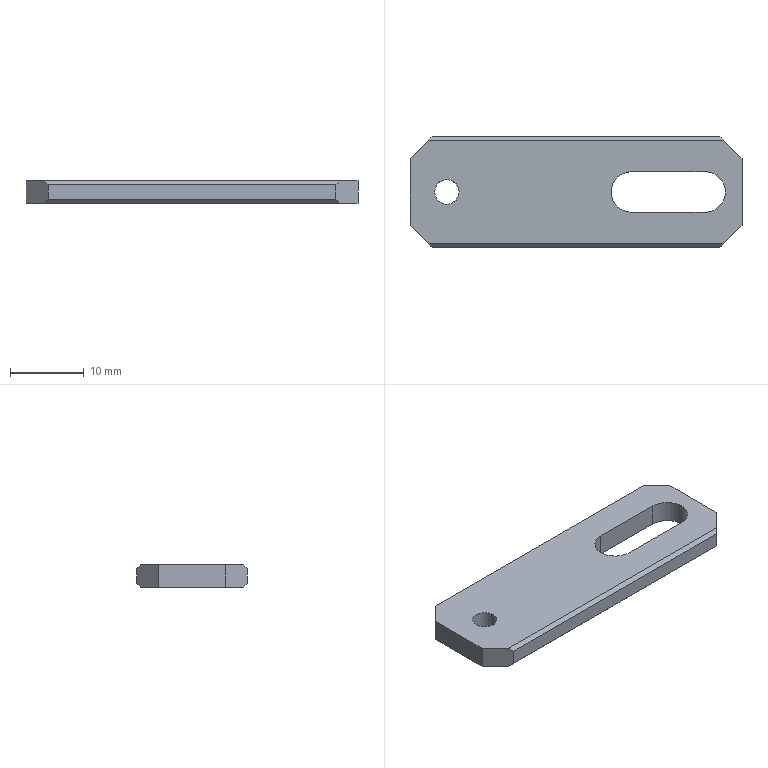Part | SolidWorks | features Chamfer 2, Extrusion 1, HoleWzd 1, ICE 1 | 1 solid | 21 faces | box 45 x 15 x 3 mm | volume 1689 mm3 | plane 16 | cylinder 5 | commonest cylinder face diameters 5.5 x3 3.3 x2
STEP:
#1=CARTESIAN_POINT('',(20.25,0.,0.));
#2=VERTEX_POINT('',#1);
#3=CARTESIAN_POINT('',(17.5,2.75,0.));
#4=VERTEX_POINT('',#3);
#5=CARTESIAN_POINT('',(17.5,0.,0.));
#6=DIRECTION('',(0.,0.,1.));
#7=DIRECTION('',(1.,0.,0.));
#8=AXIS2_PLACEMENT_3D('',#5,#6,#7);
#9=CIRCLE('',#8,2.75);
#10=EDGE_CURVE('',#2,#4,#9,.T.);
#11=ORIENTED_EDGE('',*,*,#10,.F.);
#12=CARTESIAN_POINT('',(20.25,0.,3.));
#13=VERTEX_POINT('',#12);
#14=CARTESIAN_POINT('',(20.25,0.,0.));
#15=DIRECTION('',(0.,0.,1.));
#16=VECTOR('',#15,1000.);
#17=LINE('',#14,#16);
#18=EDGE_CURVE('',#2,#13,#17,.T.);
#19=ORIENTED_EDGE('',*,*,#18,.T.);
#20=CARTESIAN_POINT('',(17.5,2.75,3.));
#21=VERTEX_POINT('',#20);
#22=CARTESIAN_POINT('',(17.5,0.,3.));
#23=DIRECTION('',(0.,0.,1.));
#24=DIRECTION('',(1.,0.,0.));
#25=AXIS2_PLACEMENT_3D('',#22,#23,#24);
#26=CIRCLE('',#25,2.75);
#27=EDGE_CURVE('',#13,#21,#26,.T.);
#28=ORIENTED_EDGE('',*,*,#27,.T.);
#29=CARTESIAN_POINT('',(17.5,2.75,0.));
#30=DIRECTION('',(0.,0.,1.));
#31=VECTOR('',#30,1000.);
#32=LINE('',#29,#31);
#33=EDGE_CURVE('',#4,#21,#32,.T.);
#34=ORIENTED_EDGE('',*,*,#33,.F.);
#35=EDGE_LOOP('',(#11,#19,#28,#34));
#36=FACE_OUTER_BOUND('',#35,.T.);
#37=CARTESIAN_POINT('',(17.5,0.,0.));
#38=DIRECTION('',(0.,0.,1.));
#39=DIRECTION('',(1.,0.,0.));
#40=AXIS2_PLACEMENT_3D('',#37,#38,#39);
#41=CYLINDRICAL_SURFACE('',#40,2.75);
#42=ADVANCED_FACE('',(#36),#41,.F.);
#43=CARTESIAN_POINT('',(-15.85,0.,0.));
#44=VERTEX_POINT('',#43);
#45=CARTESIAN_POINT('',(-19.15,0.,0.));
#46=VERTEX_POINT('',#45);
#47=CARTESIAN_POINT('',(-17.5,0.,0.));
#48=DIRECTION('',(0.,0.,-1.));
#49=DIRECTION('',(-1.,0.,0.));
#50=AXIS2_PLACEMENT_3D('',#47,#48,#49);
#51=CIRCLE('',#50,1.65);
#52=EDGE_CURVE('',#44,#46,#51,.T.);
#53=ORIENTED_EDGE('',*,*,#52,.T.);
#54=CARTESIAN_POINT('',(-19.15,0.,3.));
#55=VERTEX_POINT('',#54);
#56=CARTESIAN_POINT('',(-19.15,0.,3.));
#57=DIRECTION('',(0.,0.,1.));
#58=VECTOR('',#57,1000.);
#59=LINE('',#56,#58);
#60=EDGE_CURVE('',#46,#55,#59,.T.);
#61=ORIENTED_EDGE('',*,*,#60,.T.);
#62=CARTESIAN_POINT('',(-15.85,0.,3.));
#63=VERTEX_POINT('',#62);
#64=CARTESIAN_POINT('',(-17.5,0.,3.));
#65=DIRECTION('',(0.,0.,1.));
#66=DIRECTION('',(1.,0.,0.));
#67=AXIS2_PLACEMENT_3D('',#64,#65,#66);
#68=CIRCLE('',#67,1.65);
#69=EDGE_CURVE('',#55,#63,#68,.T.);
#70=ORIENTED_EDGE('',*,*,#69,.T.);
#71=CARTESIAN_POINT('',(-15.85,0.,3.));
#72=DIRECTION('',(0.,0.,1.));
#73=VECTOR('',#72,1000.);
#74=LINE('',#71,#73);
#75=EDGE_CURVE('',#44,#63,#74,.T.);
#76=ORIENTED_EDGE('',*,*,#75,.F.);
#77=EDGE_LOOP('',(#53,#61,#70,#76));
#78=FACE_OUTER_BOUND('',#77,.T.);
#79=CARTESIAN_POINT('',(-17.5,0.,3.));
#80=DIRECTION('',(0.,0.,1.));
#81=DIRECTION('',(1.,0.,0.));
#82=AXIS2_PLACEMENT_3D('',#79,#80,#81);
#83=CYLINDRICAL_SURFACE('',#82,1.65);
#84=ADVANCED_FACE('',(#78),#83,.F.);
#85=CARTESIAN_POINT('',(22.5,-4.5,3.));
#86=VERTEX_POINT('',#85);
#87=CARTESIAN_POINT('',(22.5,4.5,3.));
#88=VERTEX_POINT('',#87);
#89=CARTESIAN_POINT('',(22.5,-7.5,3.));
#90=DIRECTION('',(0.,1.,0.));
#91=VECTOR('',#90,1000.);
#92=LINE('',#89,#91);
#93=EDGE_CURVE('',#86,#88,#92,.T.);
#94=ORIENTED_EDGE('',*,*,#93,.F.);
#95=CARTESIAN_POINT('',(22.5,-4.5,0.));
#96=VERTEX_POINT('',#95);
#97=CARTESIAN_POINT('',(22.5,-4.5,3.));
#98=DIRECTION('',(0.,0.,-1.));
#99=VECTOR('',#98,1000.);
#100=LINE('',#97,#99);
#101=EDGE_CURVE('',#86,#96,#100,.T.);
#102=ORIENTED_EDGE('',*,*,#101,.T.);
#103=CARTESIAN_POINT('',(22.5,4.5,0.));
#104=VERTEX_POINT('',#103);
#105=CARTESIAN_POINT('',(22.5,-7.5,0.));
#106=DIRECTION('',(0.,1.,0.));
#107=VECTOR('',#106,1000.);
#108=LINE('',#105,#107);
#109=EDGE_CURVE('',#96,#104,#108,.T.);
#110=ORIENTED_EDGE('',*,*,#109,.T.);
#111=CARTESIAN_POINT('',(22.5,4.5,3.));
#112=DIRECTION('',(0.,0.,1.));
#113=VECTOR('',#112,1000.);
#114=LINE('',#111,#113);
#115=EDGE_CURVE('',#104,#88,#114,.T.);
#116=ORIENTED_EDGE('',*,*,#115,.T.);
#117=EDGE_LOOP('',(#94,#102,#110,#116));
#118=FACE_OUTER_BOUND('',#117,.T.);
#119=CARTESIAN_POINT('',(22.5,-7.5,3.));
#120=DIRECTION('',(-1.,0.,0.));
#121=DIRECTION('',(0.,0.,1.));
#122=AXIS2_PLACEMENT_3D('',#119,#120,#121);
#123=PLANE('',#122);
#124=ADVANCED_FACE('',(#118),#123,.F.);
#125=CARTESIAN_POINT('',(-19.5,7.5,0.5));
#126=VERTEX_POINT('',#125);
#127=CARTESIAN_POINT('',(-19.5,7.5,2.5));
#128=VERTEX_POINT('',#127);
#129=CARTESIAN_POINT('',(-19.5,7.5,3.));
#130=DIRECTION('',(0.,0.,1.));
#131=VECTOR('',#130,1000.);
#132=LINE('',#129,#131);
#133=EDGE_CURVE('',#126,#128,#132,.T.);
#134=ORIENTED_EDGE('',*,*,#133,.T.);
#135=CARTESIAN_POINT('',(19.5,7.5,2.5));
#136=VERTEX_POINT('',#135);
#137=CARTESIAN_POINT('',(-22.5,7.5,2.5));
#138=DIRECTION('',(1.,0.,0.));
#139=VECTOR('',#138,1000.);
#140=LINE('',#137,#139);
#141=EDGE_CURVE('',#128,#136,#140,.T.);
#142=ORIENTED_EDGE('',*,*,#141,.T.);
#143=CARTESIAN_POINT('',(19.5,7.5,0.5));
#144=VERTEX_POINT('',#143);
#145=CARTESIAN_POINT('',(19.5,7.5,3.));
#146=DIRECTION('',(0.,0.,-1.));
#147=VECTOR('',#146,1000.);
#148=LINE('',#145,#147);
#149=EDGE_CURVE('',#136,#144,#148,.T.);
#150=ORIENTED_EDGE('',*,*,#149,.T.);
#151=CARTESIAN_POINT('',(-19.5,7.5,0.5));
#152=DIRECTION('',(-1.,0.,0.));
#153=VECTOR('',#152,1000.);
#154=LINE('',#151,#153);
#155=EDGE_CURVE('',#144,#126,#154,.T.);
#156=ORIENTED_EDGE('',*,*,#155,.T.);
#157=EDGE_LOOP('',(#134,#142,#150,#156));
#158=FACE_OUTER_BOUND('',#157,.T.);
#159=CARTESIAN_POINT('',(-22.5,7.5,3.));
#160=DIRECTION('',(0.,-1.,0.));
#161=DIRECTION('',(0.,0.,-1.));
#162=AXIS2_PLACEMENT_3D('',#159,#160,#161);
#163=PLANE('',#162);
#164=ADVANCED_FACE('',(#158),#163,.F.);
#165=CARTESIAN_POINT('',(-22.5,4.5,0.));
#166=VERTEX_POINT('',#165);
#167=CARTESIAN_POINT('',(-22.5,-4.5,0.));
#168=VERTEX_POINT('',#167);
#169=CARTESIAN_POINT('',(-22.5,-7.5,0.));
#170=DIRECTION('',(0.,-1.,0.));
#171=VECTOR('',#170,1000.);
#172=LINE('',#169,#171);
#173=EDGE_CURVE('',#166,#168,#172,.T.);
#174=ORIENTED_EDGE('',*,*,#173,.T.);
#175=CARTESIAN_POINT('',(-22.5,-4.5,3.));
#176=VERTEX_POINT('',#175);
#177=CARTESIAN_POINT('',(-22.5,-4.5,3.));
#178=DIRECTION('',(0.,0.,1.));
#179=VECTOR('',#178,1000.);
#180=LINE('',#177,#179);
#181=EDGE_CURVE('',#168,#176,#180,.T.);
#182=ORIENTED_EDGE('',*,*,#181,.T.);
#183=CARTESIAN_POINT('',(-22.5,4.5,3.));
#184=VERTEX_POINT('',#183);
#185=CARTESIAN_POINT('',(-22.5,-7.5,3.));
#186=DIRECTION('',(0.,-1.,0.));
#187=VECTOR('',#186,1000.);
#188=LINE('',#185,#187);
#189=EDGE_CURVE('',#184,#176,#188,.T.);
#190=ORIENTED_EDGE('',*,*,#189,.F.);
#191=CARTESIAN_POINT('',(-22.5,4.5,3.));
#192=DIRECTION('',(0.,0.,-1.));
#193=VECTOR('',#192,1000.);
#194=LINE('',#191,#193);
#195=EDGE_CURVE('',#184,#166,#194,.T.);
#196=ORIENTED_EDGE('',*,*,#195,.T.);
#197=EDGE_LOOP('',(#174,#182,#190,#196));
#198=FACE_OUTER_BOUND('',#197,.T.);
#199=CARTESIAN_POINT('',(-22.5,-7.5,3.));
#200=DIRECTION('',(1.,0.,0.));
#201=DIRECTION('',(0.,0.,-1.));
#202=AXIS2_PLACEMENT_3D('',#199,#200,#201);
#203=PLANE('',#202);
#204=ADVANCED_FACE('',(#198),#203,.F.);
#205=CARTESIAN_POINT('',(19.5,-7.5,0.5));
#206=VERTEX_POINT('',#205);
#207=CARTESIAN_POINT('',(19.5,-7.5,2.5));
#208=VERTEX_POINT('',#207);
#209=CARTESIAN_POINT('',(19.5,-7.5,3.));
#210=DIRECTION('',(0.,0.,1.));
#211=VECTOR('',#210,1000.);
#212=LINE('',#209,#211);
#213=EDGE_CURVE('',#206,#208,#212,.T.);
#214=ORIENTED_EDGE('',*,*,#213,.T.);
#215=CARTESIAN_POINT('',(-19.5,-7.5,2.5));
#216=VERTEX_POINT('',#215);
#217=CARTESIAN_POINT('',(-22.5,-7.5,2.5));
#218=DIRECTION('',(-1.,0.,0.));
#219=VECTOR('',#218,1000.);
#220=LINE('',#217,#219);
#221=EDGE_CURVE('',#208,#216,#220,.T.);
#222=ORIENTED_EDGE('',*,*,#221,.T.);
#223=CARTESIAN_POINT('',(-19.5,-7.5,0.5));
#224=VERTEX_POINT('',#223);
#225=CARTESIAN_POINT('',(-19.5,-7.5,3.));
#226=DIRECTION('',(0.,0.,-1.));
#227=VECTOR('',#226,1000.);
#228=LINE('',#225,#227);
#229=EDGE_CURVE('',#216,#224,#228,.T.);
#230=ORIENTED_EDGE('',*,*,#229,.T.);
#231=CARTESIAN_POINT('',(19.5,-7.5,0.5));
#232=DIRECTION('',(1.,0.,0.));
#233=VECTOR('',#232,1000.);
#234=LINE('',#231,#233);
#235=EDGE_CURVE('',#224,#206,#234,.T.);
#236=ORIENTED_EDGE('',*,*,#235,.T.);
#237=EDGE_LOOP('',(#214,#222,#230,#236));
#238=FACE_OUTER_BOUND('',#237,.T.);
#239=CARTESIAN_POINT('',(-22.5,-7.5,3.));
#240=DIRECTION('',(0.,1.,0.));
#241=DIRECTION('',(0.,0.,1.));
#242=AXIS2_PLACEMENT_3D('',#239,#240,#241);
#243=PLANE('',#242);
#244=ADVANCED_FACE('',(#238),#243,.F.);
#245=CARTESIAN_POINT('',(7.5,-2.75,3.));
#246=VERTEX_POINT('',#245);
#247=CARTESIAN_POINT('',(17.5,-2.75,3.));
#248=VERTEX_POINT('',#247);
#249=CARTESIAN_POINT('',(7.5,-2.75,3.));
#250=DIRECTION('',(1.,0.,0.));
#251=VECTOR('',#250,1000.);
#252=LINE('',#249,#251);
#253=EDGE_CURVE('',#246,#248,#252,.T.);
#254=ORIENTED_EDGE('',*,*,#253,.F.);
#255=CARTESIAN_POINT('',(7.5,2.75,3.));
#256=VERTEX_POINT('',#255);
#257=CARTESIAN_POINT('',(7.5,0.,3.));
#258=DIRECTION('',(0.,0.,1.));
#259=DIRECTION('',(1.,0.,0.));
#260=AXIS2_PLACEMENT_3D('',#257,#258,#259);
#261=CIRCLE('',#260,2.75);
#262=EDGE_CURVE('',#256,#246,#261,.T.);
#263=ORIENTED_EDGE('',*,*,#262,.F.);
#264=CARTESIAN_POINT('',(7.5,2.75,3.));
#265=DIRECTION('',(-1.,0.,0.));
#266=VECTOR('',#265,1000.);
#267=LINE('',#264,#266);
#268=EDGE_CURVE('',#21,#256,#267,.T.);
#269=ORIENTED_EDGE('',*,*,#268,.F.);
#270=ORIENTED_EDGE('',*,*,#27,.F.);
#271=CARTESIAN_POINT('',(17.5,0.,3.));
#272=DIRECTION('',(0.,0.,1.));
#273=DIRECTION('',(1.,0.,0.));
#274=AXIS2_PLACEMENT_3D('',#271,#272,#273);
#275=CIRCLE('',#274,2.75);
#276=EDGE_CURVE('',#248,#13,#275,.T.);
#277=ORIENTED_EDGE('',*,*,#276,.F.);
#278=EDGE_LOOP('',(#254,#263,#269,#270,#277));
#279=FACE_BOUND('',#278,.T.);
#280=CARTESIAN_POINT('',(-17.5,0.,3.));
#281=DIRECTION('',(0.,0.,1.));
#282=DIRECTION('',(1.,0.,0.));
#283=AXIS2_PLACEMENT_3D('',#280,#281,#282);
#284=CIRCLE('',#283,1.65);
#285=EDGE_CURVE('',#63,#55,#284,.T.);
#286=ORIENTED_EDGE('',*,*,#285,.F.);
#287=ORIENTED_EDGE('',*,*,#69,.F.);
#288=EDGE_LOOP('',(#286,#287));
#289=FACE_BOUND('',#288,.T.);
#290=CARTESIAN_POINT('',(20.,7.,3.));
#291=VERTEX_POINT('',#290);
#292=CARTESIAN_POINT('',(19.5,7.5,3.));
#293=DIRECTION('',(-0.7071,0.7071,0.));
#294=VECTOR('',#293,1000.);
#295=LINE('',#292,#294);
#296=EDGE_CURVE('',#88,#291,#295,.T.);
#297=ORIENTED_EDGE('',*,*,#296,.T.);
#298=CARTESIAN_POINT('',(-20.,7.,3.));
#299=VERTEX_POINT('',#298);
#300=CARTESIAN_POINT('',(0.,7.,3.));
#301=DIRECTION('',(-1.,0.,0.));
#302=VECTOR('',#301,1000.);
#303=LINE('',#300,#302);
#304=EDGE_CURVE('',#291,#299,#303,.T.);
#305=ORIENTED_EDGE('',*,*,#304,.T.);
#306=CARTESIAN_POINT('',(-22.5,4.5,3.));
#307=DIRECTION('',(-0.7071,-0.7071,0.));
#308=VECTOR('',#307,1000.);
#309=LINE('',#306,#308);
#310=EDGE_CURVE('',#299,#184,#309,.T.);
#311=ORIENTED_EDGE('',*,*,#310,.T.);
#312=ORIENTED_EDGE('',*,*,#189,.T.);
#313=CARTESIAN_POINT('',(-20.,-7.,3.));
#314=VERTEX_POINT('',#313);
#315=CARTESIAN_POINT('',(-19.5,-7.5,3.));
#316=DIRECTION('',(0.7071,-0.7071,0.));
#317=VECTOR('',#316,1000.);
#318=LINE('',#315,#317);
#319=EDGE_CURVE('',#176,#314,#318,.T.);
#320=ORIENTED_EDGE('',*,*,#319,.T.);
#321=CARTESIAN_POINT('',(20.,-7.,3.));
#322=VERTEX_POINT('',#321);
#323=CARTESIAN_POINT('',(0.,-7.,3.));
#324=DIRECTION('',(1.,0.,0.));
#325=VECTOR('',#324,1000.);
#326=LINE('',#323,#325);
#327=EDGE_CURVE('',#314,#322,#326,.T.);
#328=ORIENTED_EDGE('',*,*,#327,.T.);
#329=CARTESIAN_POINT('',(22.5,-4.5,3.));
#330=DIRECTION('',(0.7071,0.7071,0.));
#331=VECTOR('',#330,1000.);
#332=LINE('',#329,#331);
#333=EDGE_CURVE('',#322,#86,#332,.T.);
#334=ORIENTED_EDGE('',*,*,#333,.T.);
#335=ORIENTED_EDGE('',*,*,#93,.T.);
#336=EDGE_LOOP('',(#297,#305,#311,#312,#320,#328,#334,#335));
#337=FACE_OUTER_BOUND('',#336,.T.);
#338=CARTESIAN_POINT('',(0.,0.,3.));
#339=DIRECTION('',(0.,0.,-1.));
#340=DIRECTION('',(-1.,0.,0.));
#341=AXIS2_PLACEMENT_3D('',#338,#339,#340);
#342=PLANE('',#341);
#343=ADVANCED_FACE('',(#279,#289,#337),#342,.F.);
#344=CARTESIAN_POINT('',(7.5,2.75,0.));
#345=VERTEX_POINT('',#344);
#346=CARTESIAN_POINT('',(7.5,-2.75,0.));
#347=VERTEX_POINT('',#346);
#348=CARTESIAN_POINT('',(7.5,0.,0.));
#349=DIRECTION('',(0.,0.,1.));
#350=DIRECTION('',(1.,0.,0.));
#351=AXIS2_PLACEMENT_3D('',#348,#349,#350);
#352=CIRCLE('',#351,2.75);
#353=EDGE_CURVE('',#345,#347,#352,.T.);
#354=ORIENTED_EDGE('',*,*,#353,.T.);
#355=CARTESIAN_POINT('',(17.5,-2.75,0.));
#356=VERTEX_POINT('',#355);
#357=CARTESIAN_POINT('',(7.5,-2.75,0.));
#358=DIRECTION('',(1.,0.,0.));
#359=VECTOR('',#358,1000.);
#360=LINE('',#357,#359);
#361=EDGE_CURVE('',#347,#356,#360,.T.);
#362=ORIENTED_EDGE('',*,*,#361,.T.);
#363=CARTESIAN_POINT('',(17.5,0.,0.));
#364=DIRECTION('',(0.,0.,1.));
#365=DIRECTION('',(1.,0.,0.));
#366=AXIS2_PLACEMENT_3D('',#363,#364,#365);
#367=CIRCLE('',#366,2.75);
#368=EDGE_CURVE('',#356,#2,#367,.T.);
#369=ORIENTED_EDGE('',*,*,#368,.T.);
#370=ORIENTED_EDGE('',*,*,#10,.T.);
#371=CARTESIAN_POINT('',(7.5,2.75,0.));
#372=DIRECTION('',(-1.,0.,0.));
#373=VECTOR('',#372,1000.);
#374=LINE('',#371,#373);
#375=EDGE_CURVE('',#4,#345,#374,.T.);
#376=ORIENTED_EDGE('',*,*,#375,.T.);
#377=EDGE_LOOP('',(#354,#362,#369,#370,#376));
#378=FACE_BOUND('',#377,.T.);
#379=ORIENTED_EDGE('',*,*,#52,.F.);
#380=CARTESIAN_POINT('',(-17.5,0.,0.));
#381=DIRECTION('',(0.,0.,-1.));
#382=DIRECTION('',(-1.,0.,0.));
#383=AXIS2_PLACEMENT_3D('',#380,#381,#382);
#384=CIRCLE('',#383,1.65);
#385=EDGE_CURVE('',#46,#44,#384,.T.);
#386=ORIENTED_EDGE('',*,*,#385,.F.);
#387=EDGE_LOOP('',(#379,#386));
#388=FACE_BOUND('',#387,.T.);
#389=CARTESIAN_POINT('',(-20.,7.,0.));
#390=VERTEX_POINT('',#389);
#391=CARTESIAN_POINT('',(-13.5,13.5,0.));
#392=DIRECTION('',(0.7071,0.7071,0.));
#393=VECTOR('',#392,1000.);
#394=LINE('',#391,#393);
#395=EDGE_CURVE('',#166,#390,#394,.T.);
#396=ORIENTED_EDGE('',*,*,#395,.T.);
#397=CARTESIAN_POINT('',(20.,7.,0.));
#398=VERTEX_POINT('',#397);
#399=CARTESIAN_POINT('',(19.5,7.,0.));
#400=DIRECTION('',(1.,0.,0.));
#401=VECTOR('',#400,1000.);
#402=LINE('',#399,#401);
#403=EDGE_CURVE('',#390,#398,#402,.T.);
#404=ORIENTED_EDGE('',*,*,#403,.T.);
#405=CARTESIAN_POINT('',(13.5,13.5,0.));
#406=DIRECTION('',(0.7071,-0.7071,0.));
#407=VECTOR('',#406,1000.);
#408=LINE('',#405,#407);
#409=EDGE_CURVE('',#398,#104,#408,.T.);
#410=ORIENTED_EDGE('',*,*,#409,.T.);
#411=ORIENTED_EDGE('',*,*,#109,.F.);
#412=CARTESIAN_POINT('',(20.,-7.,0.));
#413=VERTEX_POINT('',#412);
#414=CARTESIAN_POINT('',(13.5,-13.5,0.));
#415=DIRECTION('',(-0.7071,-0.7071,0.));
#416=VECTOR('',#415,1000.);
#417=LINE('',#414,#416);
#418=EDGE_CURVE('',#96,#413,#417,.T.);
#419=ORIENTED_EDGE('',*,*,#418,.T.);
#420=CARTESIAN_POINT('',(-20.,-7.,0.));
#421=VERTEX_POINT('',#420);
#422=CARTESIAN_POINT('',(-19.5,-7.,0.));
#423=DIRECTION('',(-1.,0.,0.));
#424=VECTOR('',#423,1000.);
#425=LINE('',#422,#424);
#426=EDGE_CURVE('',#413,#421,#425,.T.);
#427=ORIENTED_EDGE('',*,*,#426,.T.);
#428=CARTESIAN_POINT('',(-13.5,-13.5,0.));
#429=DIRECTION('',(-0.7071,0.7071,0.));
#430=VECTOR('',#429,1000.);
#431=LINE('',#428,#430);
#432=EDGE_CURVE('',#421,#168,#431,.T.);
#433=ORIENTED_EDGE('',*,*,#432,.T.);
#434=ORIENTED_EDGE('',*,*,#173,.F.);
#435=EDGE_LOOP('',(#396,#404,#410,#411,#419,#427,#433,#434));
#436=FACE_OUTER_BOUND('',#435,.T.);
#437=CARTESIAN_POINT('',(0.,0.,0.));
#438=DIRECTION('',(0.,0.,-1.));
#439=DIRECTION('',(-1.,0.,0.));
#440=AXIS2_PLACEMENT_3D('',#437,#438,#439);
#441=PLANE('',#440);
#442=ADVANCED_FACE('',(#378,#388,#436),#441,.T.);
#443=ORIENTED_EDGE('',*,*,#60,.F.);
#444=ORIENTED_EDGE('',*,*,#385,.T.);
#445=ORIENTED_EDGE('',*,*,#75,.T.);
#446=ORIENTED_EDGE('',*,*,#285,.T.);
#447=EDGE_LOOP('',(#443,#444,#445,#446));
#448=FACE_OUTER_BOUND('',#447,.T.);
#449=CARTESIAN_POINT('',(-17.5,0.,3.));
#450=DIRECTION('',(0.,0.,1.));
#451=DIRECTION('',(1.,0.,0.));
#452=AXIS2_PLACEMENT_3D('',#449,#450,#451);
#453=CYLINDRICAL_SURFACE('',#452,1.65);
#454=ADVANCED_FACE('',(#448),#453,.F.);
#455=ORIENTED_EDGE('',*,*,#262,.T.);
#456=CARTESIAN_POINT('',(7.5,-2.75,0.));
#457=DIRECTION('',(0.,0.,1.));
#458=VECTOR('',#457,1000.);
#459=LINE('',#456,#458);
#460=EDGE_CURVE('',#347,#246,#459,.T.);
#461=ORIENTED_EDGE('',*,*,#460,.F.);
#462=ORIENTED_EDGE('',*,*,#353,.F.);
#463=CARTESIAN_POINT('',(7.5,2.75,0.));
#464=DIRECTION('',(0.,0.,1.));
#465=VECTOR('',#464,1000.);
#466=LINE('',#463,#465);
#467=EDGE_CURVE('',#345,#256,#466,.T.);
#468=ORIENTED_EDGE('',*,*,#467,.T.);
#469=EDGE_LOOP('',(#455,#461,#462,#468));
#470=FACE_OUTER_BOUND('',#469,.T.);
#471=CARTESIAN_POINT('',(7.5,0.,0.));
#472=DIRECTION('',(0.,0.,1.));
#473=DIRECTION('',(1.,0.,0.));
#474=AXIS2_PLACEMENT_3D('',#471,#472,#473);
#475=CYLINDRICAL_SURFACE('',#474,2.75);
#476=ADVANCED_FACE('',(#470),#475,.F.);
#477=ORIENTED_EDGE('',*,*,#268,.T.);
#478=ORIENTED_EDGE('',*,*,#467,.F.);
#479=ORIENTED_EDGE('',*,*,#375,.F.);
#480=ORIENTED_EDGE('',*,*,#33,.T.);
#481=EDGE_LOOP('',(#477,#478,#479,#480));
#482=FACE_OUTER_BOUND('',#481,.T.);
#483=CARTESIAN_POINT('',(7.5,2.75,0.));
#484=DIRECTION('',(0.,1.,0.));
#485=DIRECTION('',(0.,0.,1.));
#486=AXIS2_PLACEMENT_3D('',#483,#484,#485);
#487=PLANE('',#486);
#488=ADVANCED_FACE('',(#482),#487,.F.);
#489=ORIENTED_EDGE('',*,*,#18,.F.);
#490=ORIENTED_EDGE('',*,*,#368,.F.);
#491=CARTESIAN_POINT('',(17.5,-2.75,0.));
#492=DIRECTION('',(0.,0.,1.));
#493=VECTOR('',#492,1000.);
#494=LINE('',#491,#493);
#495=EDGE_CURVE('',#356,#248,#494,.T.);
#496=ORIENTED_EDGE('',*,*,#495,.T.);
#497=ORIENTED_EDGE('',*,*,#276,.T.);
#498=EDGE_LOOP('',(#489,#490,#496,#497));
#499=FACE_OUTER_BOUND('',#498,.T.);
#500=CARTESIAN_POINT('',(17.5,0.,0.));
#501=DIRECTION('',(0.,0.,1.));
#502=DIRECTION('',(1.,0.,0.));
#503=AXIS2_PLACEMENT_3D('',#500,#501,#502);
#504=CYLINDRICAL_SURFACE('',#503,2.75);
#505=ADVANCED_FACE('',(#499),#504,.F.);
#506=ORIENTED_EDGE('',*,*,#253,.T.);
#507=ORIENTED_EDGE('',*,*,#495,.F.);
#508=ORIENTED_EDGE('',*,*,#361,.F.);
#509=ORIENTED_EDGE('',*,*,#460,.T.);
#510=EDGE_LOOP('',(#506,#507,#508,#509));
#511=FACE_OUTER_BOUND('',#510,.T.);
#512=CARTESIAN_POINT('',(7.5,-2.75,0.));
#513=DIRECTION('',(0.,-1.,0.));
#514=DIRECTION('',(0.,0.,-1.));
#515=AXIS2_PLACEMENT_3D('',#512,#513,#514);
#516=PLANE('',#515);
#517=ADVANCED_FACE('',(#511),#516,.F.);
#518=ORIENTED_EDGE('',*,*,#333,.F.);
#519=CARTESIAN_POINT('',(21.667,-5.333,4.667));
#520=DIRECTION('',(-0.5774,-0.5774,-0.5774));
#521=VECTOR('',#520,1000.);
#522=LINE('',#519,#521);
#523=EDGE_CURVE('',#322,#208,#522,.T.);
#524=ORIENTED_EDGE('',*,*,#523,.T.);
#525=ORIENTED_EDGE('',*,*,#213,.F.);
#526=CARTESIAN_POINT('',(20.667,-6.333,-0.6667));
#527=DIRECTION('',(0.5774,0.5774,-0.5774));
#528=VECTOR('',#527,1000.);
#529=LINE('',#526,#528);
#530=EDGE_CURVE('',#206,#413,#529,.T.);
#531=ORIENTED_EDGE('',*,*,#530,.T.);
#532=ORIENTED_EDGE('',*,*,#418,.F.);
#533=ORIENTED_EDGE('',*,*,#101,.F.);
#534=EDGE_LOOP('',(#518,#524,#525,#531,#532,#533));
#535=FACE_OUTER_BOUND('',#534,.T.);
#536=CARTESIAN_POINT('',(22.5,-4.5,3.));
#537=DIRECTION('',(-0.7071,0.7071,0.));
#538=DIRECTION('',(0.,0.,-1.));
#539=AXIS2_PLACEMENT_3D('',#536,#537,#538);
#540=PLANE('',#539);
#541=ADVANCED_FACE('',(#535),#540,.F.);
#542=ORIENTED_EDGE('',*,*,#149,.F.);
#543=CARTESIAN_POINT('',(19.667,7.333,2.667));
#544=DIRECTION('',(0.5774,-0.5774,0.5774));
#545=VECTOR('',#544,1000.);
#546=LINE('',#543,#545);
#547=EDGE_CURVE('',#136,#291,#546,.T.);
#548=ORIENTED_EDGE('',*,*,#547,.T.);
#549=ORIENTED_EDGE('',*,*,#296,.F.);
#550=ORIENTED_EDGE('',*,*,#115,.F.);
#551=ORIENTED_EDGE('',*,*,#409,.F.);
#552=CARTESIAN_POINT('',(18.667,8.333,1.333));
#553=DIRECTION('',(-0.5774,0.5774,0.5774));
#554=VECTOR('',#553,1000.);
#555=LINE('',#552,#554);
#556=EDGE_CURVE('',#398,#144,#555,.T.);
#557=ORIENTED_EDGE('',*,*,#556,.T.);
#558=EDGE_LOOP('',(#542,#548,#549,#550,#551,#557));
#559=FACE_OUTER_BOUND('',#558,.T.);
#560=CARTESIAN_POINT('',(19.5,7.5,3.));
#561=DIRECTION('',(-0.7071,-0.7071,0.));
#562=DIRECTION('',(0.,0.,-1.));
#563=AXIS2_PLACEMENT_3D('',#560,#561,#562);
#564=PLANE('',#563);
#565=ADVANCED_FACE('',(#559),#564,.F.);
#566=ORIENTED_EDGE('',*,*,#229,.F.);
#567=CARTESIAN_POINT('',(-19.667,-7.333,2.667));
#568=DIRECTION('',(-0.5774,0.5774,0.5774));
#569=VECTOR('',#568,1000.);
#570=LINE('',#567,#569);
#571=EDGE_CURVE('',#216,#314,#570,.T.);
#572=ORIENTED_EDGE('',*,*,#571,.T.);
#573=ORIENTED_EDGE('',*,*,#319,.F.);
#574=ORIENTED_EDGE('',*,*,#181,.F.);
#575=ORIENTED_EDGE('',*,*,#432,.F.);
#576=CARTESIAN_POINT('',(-18.667,-8.333,1.333));
#577=DIRECTION('',(0.5774,-0.5774,0.5774));
#578=VECTOR('',#577,1000.);
#579=LINE('',#576,#578);
#580=EDGE_CURVE('',#421,#224,#579,.T.);
#581=ORIENTED_EDGE('',*,*,#580,.T.);
#582=EDGE_LOOP('',(#566,#572,#573,#574,#575,#581));
#583=FACE_OUTER_BOUND('',#582,.T.);
#584=CARTESIAN_POINT('',(-19.5,-7.5,3.));
#585=DIRECTION('',(0.7071,0.7071,0.));
#586=DIRECTION('',(0.,0.,-1.));
#587=AXIS2_PLACEMENT_3D('',#584,#585,#586);
#588=PLANE('',#587);
#589=ADVANCED_FACE('',(#583),#588,.F.);
#590=ORIENTED_EDGE('',*,*,#310,.F.);
#591=CARTESIAN_POINT('',(-21.667,5.333,4.667));
#592=DIRECTION('',(0.5774,0.5774,-0.5774));
#593=VECTOR('',#592,1000.);
#594=LINE('',#591,#593);
#595=EDGE_CURVE('',#299,#128,#594,.T.);
#596=ORIENTED_EDGE('',*,*,#595,.T.);
#597=ORIENTED_EDGE('',*,*,#133,.F.);
#598=CARTESIAN_POINT('',(-20.667,6.333,-0.6667));
#599=DIRECTION('',(-0.5774,-0.5774,-0.5774));
#600=VECTOR('',#599,1000.);
#601=LINE('',#598,#600);
#602=EDGE_CURVE('',#126,#390,#601,.T.);
#603=ORIENTED_EDGE('',*,*,#602,.T.);
#604=ORIENTED_EDGE('',*,*,#395,.F.);
#605=ORIENTED_EDGE('',*,*,#195,.F.);
#606=EDGE_LOOP('',(#590,#596,#597,#603,#604,#605));
#607=FACE_OUTER_BOUND('',#606,.T.);
#608=CARTESIAN_POINT('',(-22.5,4.5,3.));
#609=DIRECTION('',(0.7071,-0.7071,0.));
#610=DIRECTION('',(0.,0.,-1.));
#611=AXIS2_PLACEMENT_3D('',#608,#609,#610);
#612=PLANE('',#611);
#613=ADVANCED_FACE('',(#607),#612,.F.);
#614=ORIENTED_EDGE('',*,*,#547,.F.);
#615=ORIENTED_EDGE('',*,*,#141,.F.);
#616=ORIENTED_EDGE('',*,*,#595,.F.);
#617=ORIENTED_EDGE('',*,*,#304,.F.);
#618=EDGE_LOOP('',(#614,#615,#616,#617));
#619=FACE_OUTER_BOUND('',#618,.T.);
#620=CARTESIAN_POINT('',(0.,7.,3.));
#621=DIRECTION('',(0.,-0.7071,-0.7071));
#622=DIRECTION('',(-1.,0.,0.));
#623=AXIS2_PLACEMENT_3D('',#620,#621,#622);
#624=PLANE('',#623);
#625=ADVANCED_FACE('',(#619),#624,.F.);
#626=ORIENTED_EDGE('',*,*,#571,.F.);
#627=ORIENTED_EDGE('',*,*,#221,.F.);
#628=ORIENTED_EDGE('',*,*,#523,.F.);
#629=ORIENTED_EDGE('',*,*,#327,.F.);
#630=EDGE_LOOP('',(#626,#627,#628,#629));
#631=FACE_OUTER_BOUND('',#630,.T.);
#632=CARTESIAN_POINT('',(0.,-7.,3.));
#633=DIRECTION('',(0.,0.7071,-0.7071));
#634=DIRECTION('',(1.,0.,0.));
#635=AXIS2_PLACEMENT_3D('',#632,#633,#634);
#636=PLANE('',#635);
#637=ADVANCED_FACE('',(#631),#636,.F.);
#638=ORIENTED_EDGE('',*,*,#556,.F.);
#639=ORIENTED_EDGE('',*,*,#403,.F.);
#640=ORIENTED_EDGE('',*,*,#602,.F.);
#641=ORIENTED_EDGE('',*,*,#155,.F.);
#642=EDGE_LOOP('',(#638,#639,#640,#641));
#643=FACE_OUTER_BOUND('',#642,.T.);
#644=CARTESIAN_POINT('',(-22.5,7.5,0.5));
#645=DIRECTION('',(0.,0.7071,-0.7071));
#646=DIRECTION('',(1.,0.,0.));
#647=AXIS2_PLACEMENT_3D('',#644,#645,#646);
#648=PLANE('',#647);
#649=ADVANCED_FACE('',(#643),#648,.T.);
#650=ORIENTED_EDGE('',*,*,#580,.F.);
#651=ORIENTED_EDGE('',*,*,#426,.F.);
#652=ORIENTED_EDGE('',*,*,#530,.F.);
#653=ORIENTED_EDGE('',*,*,#235,.F.);
#654=EDGE_LOOP('',(#650,#651,#652,#653));
#655=FACE_OUTER_BOUND('',#654,.T.);
#656=CARTESIAN_POINT('',(-22.5,-7.5,0.5));
#657=DIRECTION('',(0.,-0.7071,-0.7071));
#658=DIRECTION('',(-1.,0.,0.));
#659=AXIS2_PLACEMENT_3D('',#656,#657,#658);
#660=PLANE('',#659);
#661=ADVANCED_FACE('',(#655),#660,.T.);
#662=CLOSED_SHELL('',(#42,#84,#124,#164,#204,#244,#343,#442,#454,#476,#488,#505,#517,#541,#565,#589,#613,#625,#637,#649,#661));
#663=MANIFOLD_SOLID_BREP('',#662);
#664=CARTESIAN_POINT('',(0.,0.,0.));
#665=DIRECTION('',(0.,0.,1.));
#666=DIRECTION('',(1.,0.,0.));
#667=AXIS2_PLACEMENT_3D('',#664,#665,#666);
#668=(LENGTH_UNIT()NAMED_UNIT(*)SI_UNIT(.MILLI.,.METRE.));
#669=UNCERTAINTY_MEASURE_WITH_UNIT(LENGTH_MEASURE(0.00001),#668,'','');
#670=(NAMED_UNIT(*)PLANE_ANGLE_UNIT()SI_UNIT($,.RADIAN.));
#671=(NAMED_UNIT(*)SI_UNIT($,.STERADIAN.)SOLID_ANGLE_UNIT());
#672=(GEOMETRIC_REPRESENTATION_CONTEXT(3)GLOBAL_UNCERTAINTY_ASSIGNED_CONTEXT((#669))GLOBAL_UNIT_ASSIGNED_CONTEXT((#668,#670,#671))REPRESENTATION_CONTEXT('',''));
#673=ADVANCED_BREP_SHAPE_REPRESENTATION('',(#663,#667),#672);